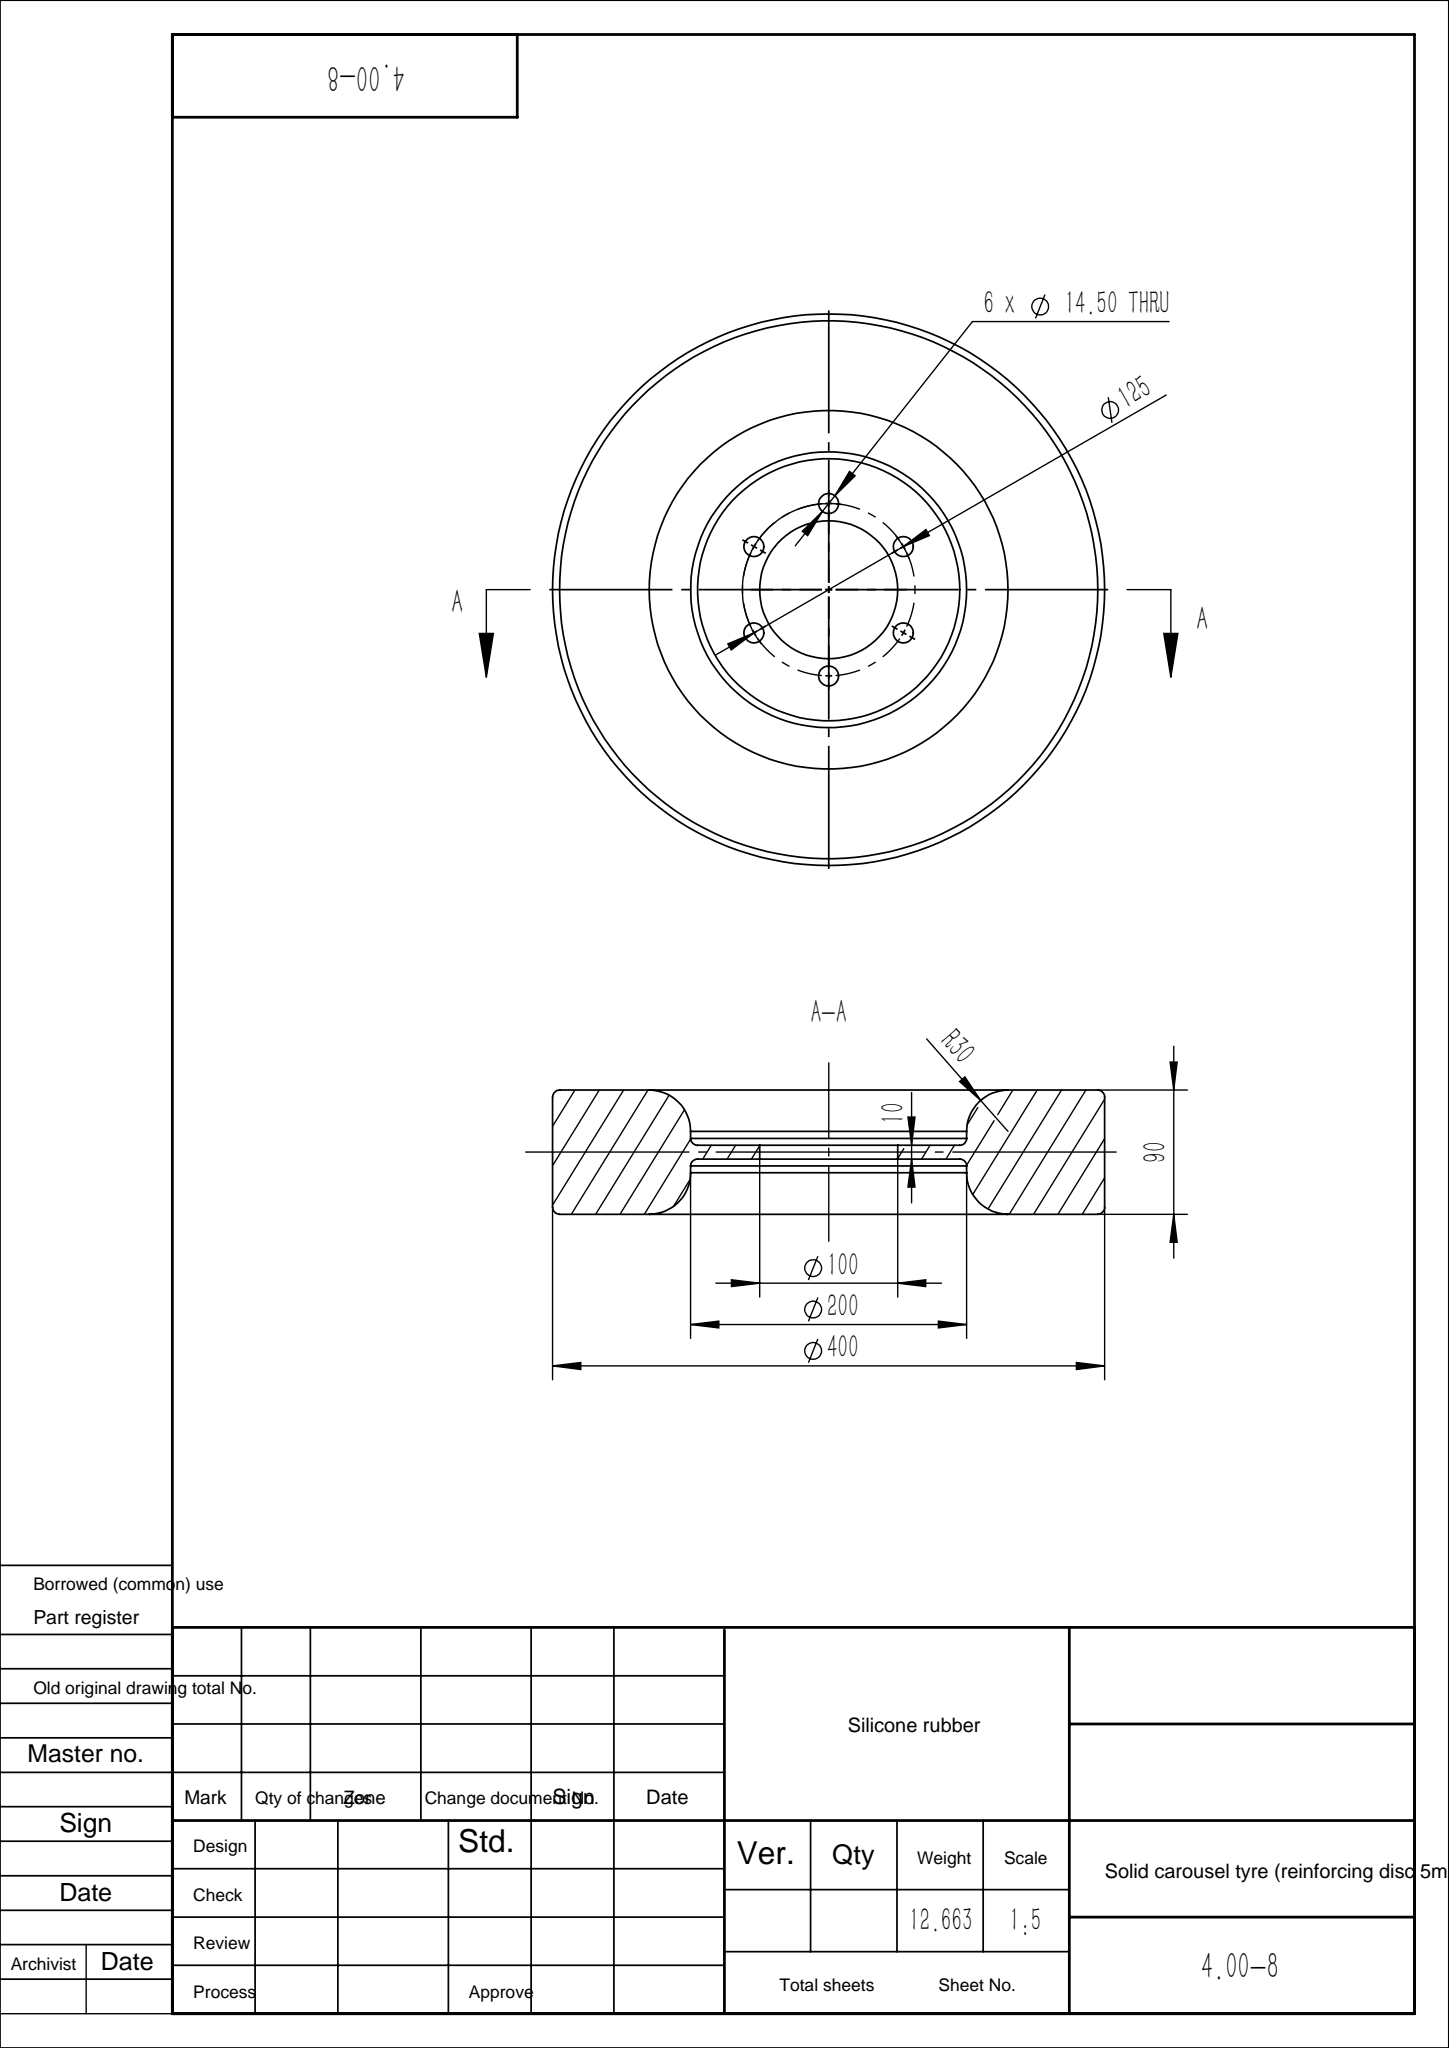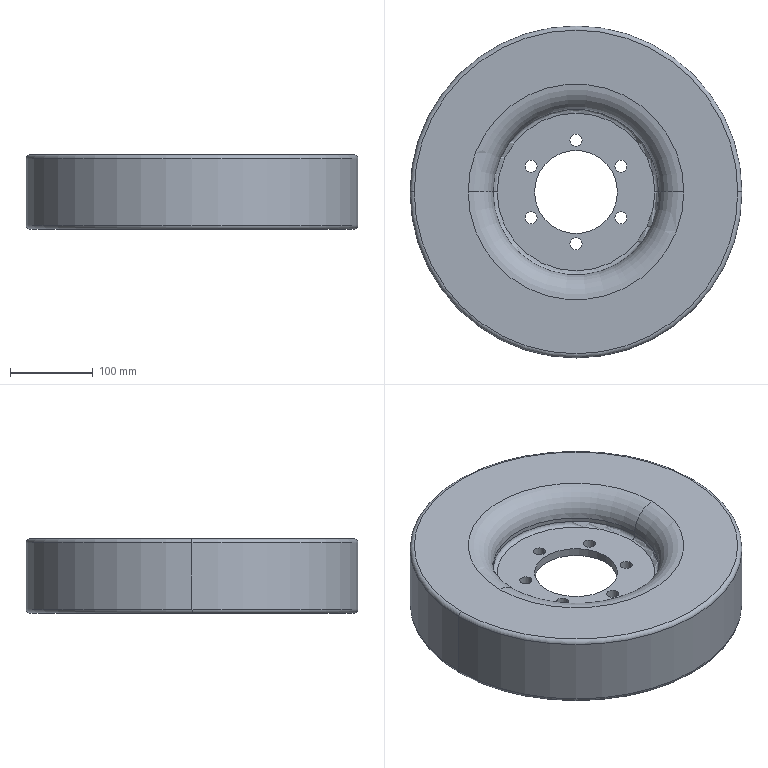Part | SolidWorks | features Fillet 1, HoleWzd 1, Revolution 1 | 1 solid | 36 faces | box 400 x 400 x 90 mm | volume 8442297 mm3 | cylinder 20 | torus 12 | plane 4 | commonest cylinder face diameters 14.5 x12 200 x4 100 x2 400 x2